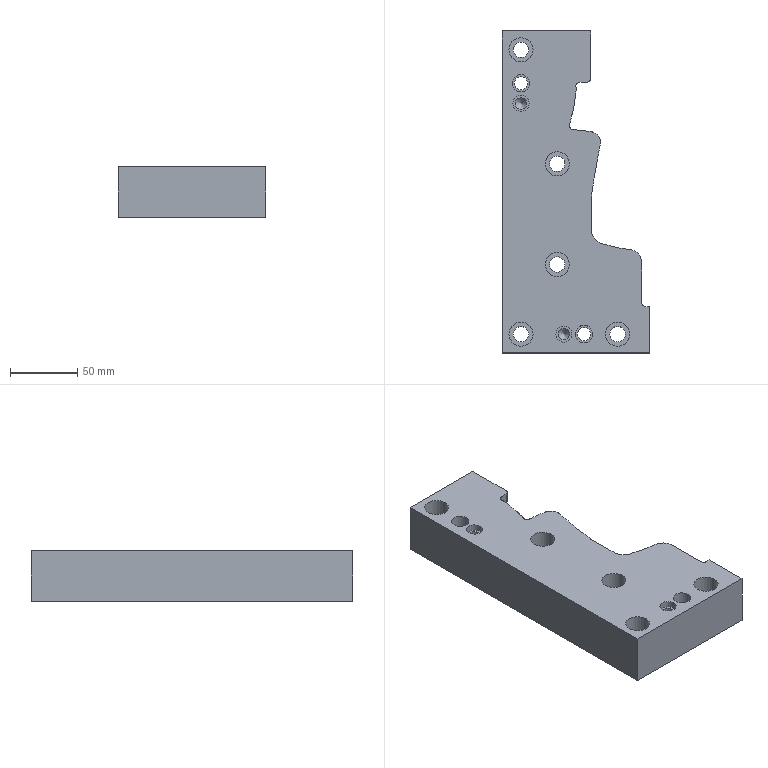Part | STEP file | lll_id4686_x_t | 1 solid | 129 faces | box 110 x 240 x 38 mm | volume 656857 mm3 | cylinder 101 | plane 26 | cone 2 | commonest cylinder face diameters 11.509 x5 18.008 x5 6 x4 13 x3 20 x3 3 x2